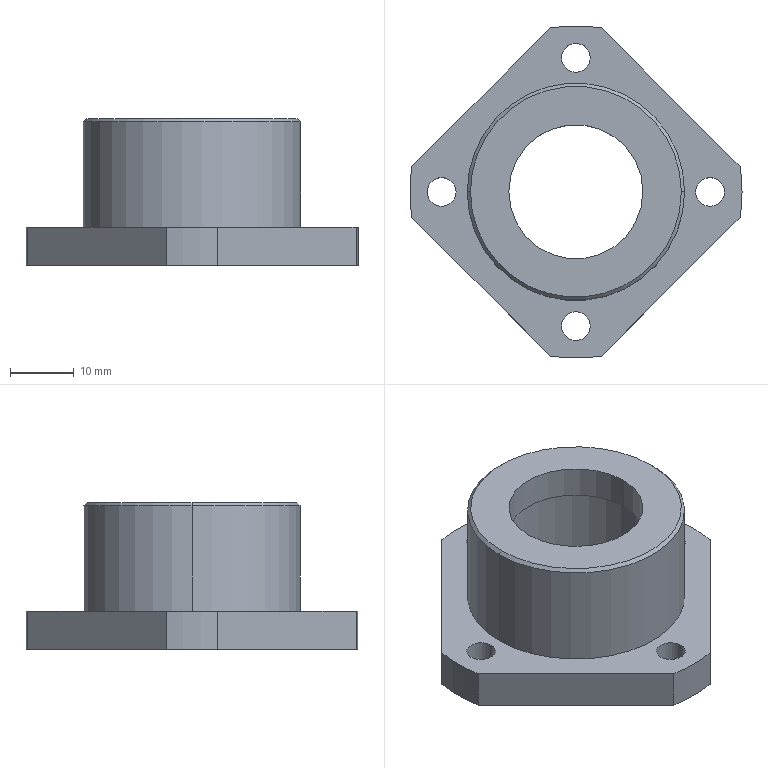Part | SolidWorks | features BaseBody 1 | 1 solid | 29 faces | box 52 x 52 x 23 mm | volume 13989 mm3 | cylinder 19 | plane 8 | cone 2 | commonest cylinder face diameters 4.5 x8 52 x5 21 x2 26 x2 34 x2
STEP:
#1=CARTESIAN_POINT('',(17.,0.,0.));
#2=VERTEX_POINT('',#1);
#3=CARTESIAN_POINT('',(-17.,0.,0.));
#4=VERTEX_POINT('',#3);
#5=CARTESIAN_POINT('',(0.,0.,0.));
#6=DIRECTION('',(0.,0.,1.));
#7=DIRECTION('',(1.,0.,0.));
#8=AXIS2_PLACEMENT_3D('',#5,#6,#7);
#9=CIRCLE('',#8,17.);
#10=EDGE_CURVE('',#2,#4,#9,.T.);
#11=ORIENTED_EDGE('',*,*,#10,.T.);
#12=CARTESIAN_POINT('',(-17.,0.,16.5));
#13=VERTEX_POINT('',#12);
#14=CARTESIAN_POINT('',(-17.,0.,-50.));
#15=DIRECTION('',(0.,0.,1.));
#16=VECTOR('',#15,1000.);
#17=LINE('',#14,#16);
#18=EDGE_CURVE('',#4,#13,#17,.T.);
#19=ORIENTED_EDGE('',*,*,#18,.T.);
#20=CARTESIAN_POINT('',(17.,0.,16.5));
#21=VERTEX_POINT('',#20);
#22=CARTESIAN_POINT('',(0.,0.,16.5));
#23=DIRECTION('',(0.,0.,-1.));
#24=DIRECTION('',(1.,0.,0.));
#25=AXIS2_PLACEMENT_3D('',#22,#23,#24);
#26=CIRCLE('',#25,17.);
#27=EDGE_CURVE('',#13,#21,#26,.T.);
#28=ORIENTED_EDGE('',*,*,#27,.T.);
#29=CARTESIAN_POINT('',(17.,0.,-50.));
#30=DIRECTION('',(0.,0.,1.));
#31=VECTOR('',#30,1000.);
#32=LINE('',#29,#31);
#33=EDGE_CURVE('',#2,#21,#32,.T.);
#34=ORIENTED_EDGE('',*,*,#33,.F.);
#35=EDGE_LOOP('',(#11,#19,#28,#34));
#36=FACE_OUTER_BOUND('',#35,.T.);
#37=CARTESIAN_POINT('',(0.,0.,-50.));
#38=DIRECTION('',(0.,0.,1.));
#39=DIRECTION('',(1.,0.,0.));
#40=AXIS2_PLACEMENT_3D('',#37,#38,#39);
#41=CYLINDRICAL_SURFACE('',#40,17.);
#42=ADVANCED_FACE('',(#36),#41,.T.);
#43=CARTESIAN_POINT('',(-16.5,0.,17.));
#44=VERTEX_POINT('',#43);
#45=CARTESIAN_POINT('',(16.5,0.,17.));
#46=VERTEX_POINT('',#45);
#47=CARTESIAN_POINT('',(0.,0.,17.));
#48=DIRECTION('',(0.,0.,-1.));
#49=DIRECTION('',(-1.,0.,0.));
#50=AXIS2_PLACEMENT_3D('',#47,#48,#49);
#51=CIRCLE('',#50,16.5);
#52=EDGE_CURVE('',#44,#46,#51,.T.);
#53=ORIENTED_EDGE('',*,*,#52,.T.);
#54=CARTESIAN_POINT('',(17.,0.,16.5));
#55=DIRECTION('',(0.7071,0.,-0.7071));
#56=VECTOR('',#55,1000.);
#57=LINE('',#54,#56);
#58=EDGE_CURVE('',#46,#21,#57,.T.);
#59=ORIENTED_EDGE('',*,*,#58,.T.);
#60=ORIENTED_EDGE('',*,*,#27,.F.);
#61=CARTESIAN_POINT('',(-17.,0.,16.5));
#62=DIRECTION('',(-0.7071,0.,-0.7071));
#63=VECTOR('',#62,1000.);
#64=LINE('',#61,#63);
#65=EDGE_CURVE('',#44,#13,#64,.T.);
#66=ORIENTED_EDGE('',*,*,#65,.F.);
#67=EDGE_LOOP('',(#53,#59,#60,#66));
#68=FACE_OUTER_BOUND('',#67,.T.);
#69=CARTESIAN_POINT('',(0.,0.,16.5));
#70=DIRECTION('',(0.,0.,-1.));
#71=DIRECTION('',(-1.,0.,0.));
#72=AXIS2_PLACEMENT_3D('',#69,#70,#71);
#73=CONICAL_SURFACE('',#72,17.,0.7854);
#74=ADVANCED_FACE('',(#68),#73,.T.);
#75=CARTESIAN_POINT('',(-2.25,-21.,0.));
#76=VERTEX_POINT('',#75);
#77=CARTESIAN_POINT('',(2.25,-21.,0.));
#78=VERTEX_POINT('',#77);
#79=CARTESIAN_POINT('',(0.,-21.,0.));
#80=DIRECTION('',(0.,0.,1.));
#81=DIRECTION('',(-1.,0.,0.));
#82=AXIS2_PLACEMENT_3D('',#79,#80,#81);
#83=CIRCLE('',#82,2.25);
#84=EDGE_CURVE('',#76,#78,#83,.T.);
#85=ORIENTED_EDGE('',*,*,#84,.T.);
#86=CARTESIAN_POINT('',(2.25,-21.,-6.));
#87=VERTEX_POINT('',#86);
#88=CARTESIAN_POINT('',(2.25,-21.,0.));
#89=DIRECTION('',(0.,0.,-1.));
#90=VECTOR('',#89,1000.);
#91=LINE('',#88,#90);
#92=EDGE_CURVE('',#78,#87,#91,.T.);
#93=ORIENTED_EDGE('',*,*,#92,.T.);
#94=CARTESIAN_POINT('',(-2.25,-21.,-6.));
#95=VERTEX_POINT('',#94);
#96=CARTESIAN_POINT('',(0.,-21.,-6.));
#97=DIRECTION('',(0.,0.,1.));
#98=DIRECTION('',(-1.,0.,0.));
#99=AXIS2_PLACEMENT_3D('',#96,#97,#98);
#100=CIRCLE('',#99,2.25);
#101=EDGE_CURVE('',#95,#87,#100,.T.);
#102=ORIENTED_EDGE('',*,*,#101,.F.);
#103=CARTESIAN_POINT('',(-2.25,-21.,0.));
#104=DIRECTION('',(0.,0.,-1.));
#105=VECTOR('',#104,1000.);
#106=LINE('',#103,#105);
#107=EDGE_CURVE('',#76,#95,#106,.T.);
#108=ORIENTED_EDGE('',*,*,#107,.F.);
#109=EDGE_LOOP('',(#85,#93,#102,#108));
#110=FACE_OUTER_BOUND('',#109,.T.);
#111=CARTESIAN_POINT('',(0.,-21.,0.));
#112=DIRECTION('',(0.,0.,-1.));
#113=DIRECTION('',(-1.,0.,0.));
#114=AXIS2_PLACEMENT_3D('',#111,#112,#113);
#115=CYLINDRICAL_SURFACE('',#114,2.25);
#116=ADVANCED_FACE('',(#110),#115,.F.);
#117=CARTESIAN_POINT('',(18.75,0.,0.));
#118=VERTEX_POINT('',#117);
#119=CARTESIAN_POINT('',(23.25,0.,0.));
#120=VERTEX_POINT('',#119);
#121=CARTESIAN_POINT('',(21.,0.,0.));
#122=DIRECTION('',(0.,0.,1.));
#123=DIRECTION('',(-1.,0.,0.));
#124=AXIS2_PLACEMENT_3D('',#121,#122,#123);
#125=CIRCLE('',#124,2.25);
#126=EDGE_CURVE('',#118,#120,#125,.T.);
#127=ORIENTED_EDGE('',*,*,#126,.T.);
#128=CARTESIAN_POINT('',(23.25,0.,-6.));
#129=VERTEX_POINT('',#128);
#130=CARTESIAN_POINT('',(23.25,0.,0.));
#131=DIRECTION('',(0.,0.,-1.));
#132=VECTOR('',#131,1000.);
#133=LINE('',#130,#132);
#134=EDGE_CURVE('',#120,#129,#133,.T.);
#135=ORIENTED_EDGE('',*,*,#134,.T.);
#136=CARTESIAN_POINT('',(18.75,0.,-6.));
#137=VERTEX_POINT('',#136);
#138=CARTESIAN_POINT('',(21.,0.,-6.));
#139=DIRECTION('',(0.,0.,1.));
#140=DIRECTION('',(-1.,0.,0.));
#141=AXIS2_PLACEMENT_3D('',#138,#139,#140);
#142=CIRCLE('',#141,2.25);
#143=EDGE_CURVE('',#137,#129,#142,.T.);
#144=ORIENTED_EDGE('',*,*,#143,.F.);
#145=CARTESIAN_POINT('',(18.75,0.,0.));
#146=DIRECTION('',(0.,0.,-1.));
#147=VECTOR('',#146,1000.);
#148=LINE('',#145,#147);
#149=EDGE_CURVE('',#118,#137,#148,.T.);
#150=ORIENTED_EDGE('',*,*,#149,.F.);
#151=EDGE_LOOP('',(#127,#135,#144,#150));
#152=FACE_OUTER_BOUND('',#151,.T.);
#153=CARTESIAN_POINT('',(21.,0.,0.));
#154=DIRECTION('',(0.,0.,-1.));
#155=DIRECTION('',(-1.,0.,0.));
#156=AXIS2_PLACEMENT_3D('',#153,#154,#155);
#157=CYLINDRICAL_SURFACE('',#156,2.25);
#158=ADVANCED_FACE('',(#152),#157,.F.);
#159=CARTESIAN_POINT('',(-23.25,0.,-6.));
#160=VERTEX_POINT('',#159);
#161=CARTESIAN_POINT('',(-18.75,0.,-6.));
#162=VERTEX_POINT('',#161);
#163=CARTESIAN_POINT('',(-21.,0.,-6.));
#164=DIRECTION('',(0.,0.,1.));
#165=DIRECTION('',(1.,0.,0.));
#166=AXIS2_PLACEMENT_3D('',#163,#164,#165);
#167=CIRCLE('',#166,2.25);
#168=EDGE_CURVE('',#160,#162,#167,.T.);
#169=ORIENTED_EDGE('',*,*,#168,.F.);
#170=CARTESIAN_POINT('',(-23.25,0.,0.));
#171=VERTEX_POINT('',#170);
#172=CARTESIAN_POINT('',(-23.25,0.,-10.));
#173=DIRECTION('',(0.,0.,1.));
#174=VECTOR('',#173,1000.);
#175=LINE('',#172,#174);
#176=EDGE_CURVE('',#160,#171,#175,.T.);
#177=ORIENTED_EDGE('',*,*,#176,.T.);
#178=CARTESIAN_POINT('',(-18.75,0.,0.));
#179=VERTEX_POINT('',#178);
#180=CARTESIAN_POINT('',(-21.,0.,0.));
#181=DIRECTION('',(0.,0.,1.));
#182=DIRECTION('',(1.,0.,0.));
#183=AXIS2_PLACEMENT_3D('',#180,#181,#182);
#184=CIRCLE('',#183,2.25);
#185=EDGE_CURVE('',#171,#179,#184,.T.);
#186=ORIENTED_EDGE('',*,*,#185,.T.);
#187=CARTESIAN_POINT('',(-18.75,0.,-10.));
#188=DIRECTION('',(0.,0.,1.));
#189=VECTOR('',#188,1000.);
#190=LINE('',#187,#189);
#191=EDGE_CURVE('',#162,#179,#190,.T.);
#192=ORIENTED_EDGE('',*,*,#191,.F.);
#193=EDGE_LOOP('',(#169,#177,#186,#192));
#194=FACE_OUTER_BOUND('',#193,.T.);
#195=CARTESIAN_POINT('',(-21.,0.,-10.));
#196=DIRECTION('',(0.,0.,1.));
#197=DIRECTION('',(1.,0.,0.));
#198=AXIS2_PLACEMENT_3D('',#195,#196,#197);
#199=CYLINDRICAL_SURFACE('',#198,2.25);
#200=ADVANCED_FACE('',(#194),#199,.F.);
#201=CARTESIAN_POINT('',(-2.25,21.,-6.));
#202=VERTEX_POINT('',#201);
#203=CARTESIAN_POINT('',(2.25,21.,-6.));
#204=VERTEX_POINT('',#203);
#205=CARTESIAN_POINT('',(0.,21.,-6.));
#206=DIRECTION('',(0.,0.,1.));
#207=DIRECTION('',(1.,0.,0.));
#208=AXIS2_PLACEMENT_3D('',#205,#206,#207);
#209=CIRCLE('',#208,2.25);
#210=EDGE_CURVE('',#202,#204,#209,.T.);
#211=ORIENTED_EDGE('',*,*,#210,.F.);
#212=CARTESIAN_POINT('',(-2.25,21.,0.));
#213=VERTEX_POINT('',#212);
#214=CARTESIAN_POINT('',(-2.25,21.,-10.));
#215=DIRECTION('',(0.,0.,1.));
#216=VECTOR('',#215,1000.);
#217=LINE('',#214,#216);
#218=EDGE_CURVE('',#202,#213,#217,.T.);
#219=ORIENTED_EDGE('',*,*,#218,.T.);
#220=CARTESIAN_POINT('',(2.25,21.,0.));
#221=VERTEX_POINT('',#220);
#222=CARTESIAN_POINT('',(0.,21.,0.));
#223=DIRECTION('',(0.,0.,1.));
#224=DIRECTION('',(1.,0.,0.));
#225=AXIS2_PLACEMENT_3D('',#222,#223,#224);
#226=CIRCLE('',#225,2.25);
#227=EDGE_CURVE('',#213,#221,#226,.T.);
#228=ORIENTED_EDGE('',*,*,#227,.T.);
#229=CARTESIAN_POINT('',(2.25,21.,-10.));
#230=DIRECTION('',(0.,0.,1.));
#231=VECTOR('',#230,1000.);
#232=LINE('',#229,#231);
#233=EDGE_CURVE('',#204,#221,#232,.T.);
#234=ORIENTED_EDGE('',*,*,#233,.F.);
#235=EDGE_LOOP('',(#211,#219,#228,#234));
#236=FACE_OUTER_BOUND('',#235,.T.);
#237=CARTESIAN_POINT('',(0.,21.,-10.));
#238=DIRECTION('',(0.,0.,1.));
#239=DIRECTION('',(1.,0.,0.));
#240=AXIS2_PLACEMENT_3D('',#237,#238,#239);
#241=CYLINDRICAL_SURFACE('',#240,2.25);
#242=ADVANCED_FACE('',(#236),#241,.F.);
#243=CARTESIAN_POINT('',(25.689,-4.01,-6.));
#244=VERTEX_POINT('',#243);
#245=CARTESIAN_POINT('',(26.,0.,-6.));
#246=VERTEX_POINT('',#245);
#247=CARTESIAN_POINT('',(0.,0.,-6.));
#248=DIRECTION('',(0.,0.,1.));
#249=DIRECTION('',(1.,0.,0.));
#250=AXIS2_PLACEMENT_3D('',#247,#248,#249);
#251=CIRCLE('',#250,26.);
#252=EDGE_CURVE('',#244,#246,#251,.T.);
#253=ORIENTED_EDGE('',*,*,#252,.T.);
#254=CARTESIAN_POINT('',(26.,0.,0.));
#255=VERTEX_POINT('',#254);
#256=CARTESIAN_POINT('',(26.,0.,-50.));
#257=DIRECTION('',(0.,0.,1.));
#258=VECTOR('',#257,1000.);
#259=LINE('',#256,#258);
#260=EDGE_CURVE('',#246,#255,#259,.T.);
#261=ORIENTED_EDGE('',*,*,#260,.T.);
#262=CARTESIAN_POINT('',(25.689,-4.01,0.));
#263=VERTEX_POINT('',#262);
#264=CARTESIAN_POINT('',(0.,0.,0.));
#265=DIRECTION('',(0.,0.,-1.));
#266=DIRECTION('',(1.,0.,0.));
#267=AXIS2_PLACEMENT_3D('',#264,#265,#266);
#268=CIRCLE('',#267,26.);
#269=EDGE_CURVE('',#255,#263,#268,.T.);
#270=ORIENTED_EDGE('',*,*,#269,.T.);
#271=CARTESIAN_POINT('',(25.689,-4.01,-10.));
#272=DIRECTION('',(0.,0.,-1.));
#273=VECTOR('',#272,1000.);
#274=LINE('',#271,#273);
#275=EDGE_CURVE('',#263,#244,#274,.T.);
#276=ORIENTED_EDGE('',*,*,#275,.T.);
#277=EDGE_LOOP('',(#253,#261,#270,#276));
#278=FACE_OUTER_BOUND('',#277,.T.);
#279=CARTESIAN_POINT('',(0.,0.,-50.));
#280=DIRECTION('',(0.,0.,1.));
#281=DIRECTION('',(1.,0.,0.));
#282=AXIS2_PLACEMENT_3D('',#279,#280,#281);
#283=CYLINDRICAL_SURFACE('',#282,26.);
#284=ADVANCED_FACE('',(#278),#283,.T.);
#285=CARTESIAN_POINT('',(-10.5,0.,12.));
#286=VERTEX_POINT('',#285);
#287=CARTESIAN_POINT('',(10.5,0.,12.));
#288=VERTEX_POINT('',#287);
#289=CARTESIAN_POINT('',(0.,0.,12.));
#290=DIRECTION('',(0.,0.,1.));
#291=DIRECTION('',(1.,0.,0.));
#292=AXIS2_PLACEMENT_3D('',#289,#290,#291);
#293=CIRCLE('',#292,10.5);
#294=EDGE_CURVE('',#286,#288,#293,.T.);
#295=ORIENTED_EDGE('',*,*,#294,.F.);
#296=CARTESIAN_POINT('',(-10.5,0.,17.));
#297=VERTEX_POINT('',#296);
#298=CARTESIAN_POINT('',(-10.5,0.,-50.));
#299=DIRECTION('',(0.,0.,1.));
#300=VECTOR('',#299,1000.);
#301=LINE('',#298,#300);
#302=EDGE_CURVE('',#286,#297,#301,.T.);
#303=ORIENTED_EDGE('',*,*,#302,.T.);
#304=CARTESIAN_POINT('',(10.5,0.,17.));
#305=VERTEX_POINT('',#304);
#306=CARTESIAN_POINT('',(0.,0.,17.));
#307=DIRECTION('',(0.,0.,1.));
#308=DIRECTION('',(1.,0.,0.));
#309=AXIS2_PLACEMENT_3D('',#306,#307,#308);
#310=CIRCLE('',#309,10.5);
#311=EDGE_CURVE('',#297,#305,#310,.T.);
#312=ORIENTED_EDGE('',*,*,#311,.T.);
#313=CARTESIAN_POINT('',(10.5,0.,-50.));
#314=DIRECTION('',(0.,0.,1.));
#315=VECTOR('',#314,1000.);
#316=LINE('',#313,#315);
#317=EDGE_CURVE('',#288,#305,#316,.T.);
#318=ORIENTED_EDGE('',*,*,#317,.F.);
#319=EDGE_LOOP('',(#295,#303,#312,#318));
#320=FACE_OUTER_BOUND('',#319,.T.);
#321=CARTESIAN_POINT('',(0.,0.,-50.));
#322=DIRECTION('',(0.,0.,1.));
#323=DIRECTION('',(1.,0.,0.));
#324=AXIS2_PLACEMENT_3D('',#321,#322,#323);
#325=CYLINDRICAL_SURFACE('',#324,10.5);
#326=ADVANCED_FACE('',(#320),#325,.F.);
#327=CARTESIAN_POINT('',(-13.,0.,-6.));
#328=VERTEX_POINT('',#327);
#329=CARTESIAN_POINT('',(13.,0.,-6.));
#330=VERTEX_POINT('',#329);
#331=CARTESIAN_POINT('',(0.,0.,-6.));
#332=DIRECTION('',(0.,0.,1.));
#333=DIRECTION('',(1.,0.,0.));
#334=AXIS2_PLACEMENT_3D('',#331,#332,#333);
#335=CIRCLE('',#334,13.);
#336=EDGE_CURVE('',#328,#330,#335,.T.);
#337=ORIENTED_EDGE('',*,*,#336,.F.);
#338=CARTESIAN_POINT('',(-13.,0.,12.));
#339=VERTEX_POINT('',#338);
#340=CARTESIAN_POINT('',(-13.,0.,-17.5));
#341=DIRECTION('',(0.,0.,1.));
#342=VECTOR('',#341,1000.);
#343=LINE('',#340,#342);
#344=EDGE_CURVE('',#328,#339,#343,.T.);
#345=ORIENTED_EDGE('',*,*,#344,.T.);
#346=CARTESIAN_POINT('',(13.,0.,12.));
#347=VERTEX_POINT('',#346);
#348=CARTESIAN_POINT('',(0.,0.,12.));
#349=DIRECTION('',(0.,0.,-1.));
#350=DIRECTION('',(1.,0.,0.));
#351=AXIS2_PLACEMENT_3D('',#348,#349,#350);
#352=CIRCLE('',#351,13.);
#353=EDGE_CURVE('',#347,#339,#352,.T.);
#354=ORIENTED_EDGE('',*,*,#353,.F.);
#355=CARTESIAN_POINT('',(13.,0.,-17.5));
#356=DIRECTION('',(0.,0.,1.));
#357=VECTOR('',#356,1000.);
#358=LINE('',#355,#357);
#359=EDGE_CURVE('',#330,#347,#358,.T.);
#360=ORIENTED_EDGE('',*,*,#359,.F.);
#361=EDGE_LOOP('',(#337,#345,#354,#360));
#362=FACE_OUTER_BOUND('',#361,.T.);
#363=CARTESIAN_POINT('',(0.,0.,-17.5));
#364=DIRECTION('',(0.,0.,1.));
#365=DIRECTION('',(1.,0.,0.));
#366=AXIS2_PLACEMENT_3D('',#363,#364,#365);
#367=CYLINDRICAL_SURFACE('',#366,13.);
#368=ADVANCED_FACE('',(#362),#367,.F.);
#369=ORIENTED_EDGE('',*,*,#18,.F.);
#370=CARTESIAN_POINT('',(0.,0.,0.));
#371=DIRECTION('',(0.,0.,1.));
#372=DIRECTION('',(1.,0.,0.));
#373=AXIS2_PLACEMENT_3D('',#370,#371,#372);
#374=CIRCLE('',#373,17.);
#375=EDGE_CURVE('',#4,#2,#374,.T.);
#376=ORIENTED_EDGE('',*,*,#375,.T.);
#377=ORIENTED_EDGE('',*,*,#33,.T.);
#378=CARTESIAN_POINT('',(0.,0.,16.5));
#379=DIRECTION('',(0.,0.,-1.));
#380=DIRECTION('',(1.,0.,0.));
#381=AXIS2_PLACEMENT_3D('',#378,#379,#380);
#382=CIRCLE('',#381,17.);
#383=EDGE_CURVE('',#21,#13,#382,.T.);
#384=ORIENTED_EDGE('',*,*,#383,.T.);
#385=EDGE_LOOP('',(#369,#376,#377,#384));
#386=FACE_OUTER_BOUND('',#385,.T.);
#387=CARTESIAN_POINT('',(0.,0.,-50.));
#388=DIRECTION('',(0.,0.,1.));
#389=DIRECTION('',(1.,0.,0.));
#390=AXIS2_PLACEMENT_3D('',#387,#388,#389);
#391=CYLINDRICAL_SURFACE('',#390,17.);
#392=ADVANCED_FACE('',(#386),#391,.T.);
#393=ORIENTED_EDGE('',*,*,#58,.F.);
#394=CARTESIAN_POINT('',(0.,0.,17.));
#395=DIRECTION('',(0.,0.,-1.));
#396=DIRECTION('',(-1.,0.,0.));
#397=AXIS2_PLACEMENT_3D('',#394,#395,#396);
#398=CIRCLE('',#397,16.5);
#399=EDGE_CURVE('',#46,#44,#398,.T.);
#400=ORIENTED_EDGE('',*,*,#399,.T.);
#401=ORIENTED_EDGE('',*,*,#65,.T.);
#402=ORIENTED_EDGE('',*,*,#383,.F.);
#403=EDGE_LOOP('',(#393,#400,#401,#402));
#404=FACE_OUTER_BOUND('',#403,.T.);
#405=CARTESIAN_POINT('',(0.,0.,16.5));
#406=DIRECTION('',(0.,0.,-1.));
#407=DIRECTION('',(-1.,0.,0.));
#408=AXIS2_PLACEMENT_3D('',#405,#406,#407);
#409=CONICAL_SURFACE('',#408,17.,0.7854);
#410=ADVANCED_FACE('',(#404),#409,.T.);
#411=ORIENTED_EDGE('',*,*,#10,.F.);
#412=ORIENTED_EDGE('',*,*,#375,.F.);
#413=EDGE_LOOP('',(#411,#412));
#414=FACE_BOUND('',#413,.T.);
#415=ORIENTED_EDGE('',*,*,#84,.F.);
#416=CARTESIAN_POINT('',(0.,-21.,0.));
#417=DIRECTION('',(0.,0.,1.));
#418=DIRECTION('',(-1.,0.,0.));
#419=AXIS2_PLACEMENT_3D('',#416,#417,#418);
#420=CIRCLE('',#419,2.25);
#421=EDGE_CURVE('',#78,#76,#420,.T.);
#422=ORIENTED_EDGE('',*,*,#421,.F.);
#423=EDGE_LOOP('',(#415,#422));
#424=FACE_BOUND('',#423,.T.);
#425=ORIENTED_EDGE('',*,*,#126,.F.);
#426=CARTESIAN_POINT('',(21.,0.,0.));
#427=DIRECTION('',(0.,0.,1.));
#428=DIRECTION('',(-1.,0.,0.));
#429=AXIS2_PLACEMENT_3D('',#426,#427,#428);
#430=CIRCLE('',#429,2.25);
#431=EDGE_CURVE('',#120,#118,#430,.T.);
#432=ORIENTED_EDGE('',*,*,#431,.F.);
#433=EDGE_LOOP('',(#425,#432));
#434=FACE_BOUND('',#433,.T.);
#435=CARTESIAN_POINT('',(-21.,0.,0.));
#436=DIRECTION('',(0.,0.,1.));
#437=DIRECTION('',(1.,0.,0.));
#438=AXIS2_PLACEMENT_3D('',#435,#436,#437);
#439=CIRCLE('',#438,2.25);
#440=EDGE_CURVE('',#179,#171,#439,.T.);
#441=ORIENTED_EDGE('',*,*,#440,.F.);
#442=ORIENTED_EDGE('',*,*,#185,.F.);
#443=EDGE_LOOP('',(#441,#442));
#444=FACE_BOUND('',#443,.T.);
#445=CARTESIAN_POINT('',(0.,21.,0.));
#446=DIRECTION('',(0.,0.,1.));
#447=DIRECTION('',(1.,0.,0.));
#448=AXIS2_PLACEMENT_3D('',#445,#446,#447);
#449=CIRCLE('',#448,2.25);
#450=EDGE_CURVE('',#221,#213,#449,.T.);
#451=ORIENTED_EDGE('',*,*,#450,.F.);
#452=ORIENTED_EDGE('',*,*,#227,.F.);
#453=EDGE_LOOP('',(#451,#452));
#454=FACE_BOUND('',#453,.T.);
#455=CARTESIAN_POINT('',(-25.689,4.01,0.));
#456=VERTEX_POINT('',#455);
#457=CARTESIAN_POINT('',(-4.01,25.689,0.));
#458=VERTEX_POINT('',#457);
#459=CARTESIAN_POINT('',(-25.689,4.01,0.));
#460=DIRECTION('',(0.7071,0.7071,0.));
#461=VECTOR('',#460,1000.);
#462=LINE('',#459,#461);
#463=EDGE_CURVE('',#456,#458,#462,.T.);
#464=ORIENTED_EDGE('',*,*,#463,.F.);
#465=CARTESIAN_POINT('',(-25.689,-4.01,0.));
#466=VERTEX_POINT('',#465);
#467=CARTESIAN_POINT('',(0.,0.,0.));
#468=DIRECTION('',(0.,0.,-1.));
#469=DIRECTION('',(1.,0.,0.));
#470=AXIS2_PLACEMENT_3D('',#467,#468,#469);
#471=CIRCLE('',#470,26.);
#472=EDGE_CURVE('',#466,#456,#471,.T.);
#473=ORIENTED_EDGE('',*,*,#472,.F.);
#474=CARTESIAN_POINT('',(-4.01,-25.689,0.));
#475=VERTEX_POINT('',#474);
#476=CARTESIAN_POINT('',(-4.01,-25.689,0.));
#477=DIRECTION('',(-0.7071,0.7071,0.));
#478=VECTOR('',#477,1000.);
#479=LINE('',#476,#478);
#480=EDGE_CURVE('',#475,#466,#479,.T.);
#481=ORIENTED_EDGE('',*,*,#480,.F.);
#482=CARTESIAN_POINT('',(4.01,-25.689,0.));
#483=VERTEX_POINT('',#482);
#484=CARTESIAN_POINT('',(0.,0.,0.));
#485=DIRECTION('',(0.,0.,-1.));
#486=DIRECTION('',(1.,0.,0.));
#487=AXIS2_PLACEMENT_3D('',#484,#485,#486);
#488=CIRCLE('',#487,26.);
#489=EDGE_CURVE('',#483,#475,#488,.T.);
#490=ORIENTED_EDGE('',*,*,#489,.F.);
#491=CARTESIAN_POINT('',(25.689,-4.01,0.));
#492=DIRECTION('',(-0.7071,-0.7071,0.));
#493=VECTOR('',#492,1000.);
#494=LINE('',#491,#493);
#495=EDGE_CURVE('',#263,#483,#494,.T.);
#496=ORIENTED_EDGE('',*,*,#495,.F.);
#497=ORIENTED_EDGE('',*,*,#269,.F.);
#498=CARTESIAN_POINT('',(25.689,4.01,0.));
#499=VERTEX_POINT('',#498);
#500=CARTESIAN_POINT('',(0.,0.,0.));
#501=DIRECTION('',(0.,0.,-1.));
#502=DIRECTION('',(1.,0.,0.));
#503=AXIS2_PLACEMENT_3D('',#500,#501,#502);
#504=CIRCLE('',#503,26.);
#505=EDGE_CURVE('',#499,#255,#504,.T.);
#506=ORIENTED_EDGE('',*,*,#505,.F.);
#507=CARTESIAN_POINT('',(4.01,25.689,0.));
#508=VERTEX_POINT('',#507);
#509=CARTESIAN_POINT('',(4.01,25.689,0.));
#510=DIRECTION('',(0.7071,-0.7071,0.));
#511=VECTOR('',#510,1000.);
#512=LINE('',#509,#511);
#513=EDGE_CURVE('',#508,#499,#512,.T.);
#514=ORIENTED_EDGE('',*,*,#513,.F.);
#515=CARTESIAN_POINT('',(0.,0.,0.));
#516=DIRECTION('',(0.,0.,-1.));
#517=DIRECTION('',(1.,0.,0.));
#518=AXIS2_PLACEMENT_3D('',#515,#516,#517);
#519=CIRCLE('',#518,26.);
#520=EDGE_CURVE('',#458,#508,#519,.T.);
#521=ORIENTED_EDGE('',*,*,#520,.F.);
#522=EDGE_LOOP('',(#464,#473,#481,#490,#496,#497,#506,#514,#521));
#523=FACE_OUTER_BOUND('',#522,.T.);
#524=CARTESIAN_POINT('',(0.,17.,0.));
#525=DIRECTION('',(0.,0.,-1.));
#526=DIRECTION('',(-1.,0.,0.));
#527=AXIS2_PLACEMENT_3D('',#524,#525,#526);
#528=PLANE('',#527);
#529=ADVANCED_FACE('',(#414,#424,#434,#444,#454,#523),#528,.F.);
#530=CARTESIAN_POINT('',(0.,0.,17.));
#531=DIRECTION('',(0.,0.,1.));
#532=DIRECTION('',(1.,0.,0.));
#533=AXIS2_PLACEMENT_3D('',#530,#531,#532);
#534=CIRCLE('',#533,10.5);
#535=EDGE_CURVE('',#305,#297,#534,.T.);
#536=ORIENTED_EDGE('',*,*,#535,.F.);
#537=ORIENTED_EDGE('',*,*,#311,.F.);
#538=EDGE_LOOP('',(#536,#537));
#539=FACE_BOUND('',#538,.T.);
#540=ORIENTED_EDGE('',*,*,#52,.F.);
#541=ORIENTED_EDGE('',*,*,#399,.F.);
#542=EDGE_LOOP('',(#540,#541));
#543=FACE_OUTER_BOUND('',#542,.T.);
#544=CARTESIAN_POINT('',(0.,10.5,17.));
#545=DIRECTION('',(0.,0.,-1.));
#546=DIRECTION('',(-1.,0.,0.));
#547=AXIS2_PLACEMENT_3D('',#544,#545,#546);
#548=PLANE('',#547);
#549=ADVANCED_FACE('',(#539,#543),#548,.F.);
#550=ORIENTED_EDGE('',*,*,#92,.F.);
#551=ORIENTED_EDGE('',*,*,#421,.T.);
#552=ORIENTED_EDGE('',*,*,#107,.T.);
#553=CARTESIAN_POINT('',(0.,-21.,-6.));
#554=DIRECTION('',(0.,0.,1.));
#555=DIRECTION('',(-1.,0.,0.));
#556=AXIS2_PLACEMENT_3D('',#553,#554,#555);
#557=CIRCLE('',#556,2.25);
#558=EDGE_CURVE('',#87,#95,#557,.T.);
#559=ORIENTED_EDGE('',*,*,#558,.F.);
#560=EDGE_LOOP('',(#550,#551,#552,#559));
#561=FACE_OUTER_BOUND('',#560,.T.);
#562=CARTESIAN_POINT('',(0.,-21.,0.));
#563=DIRECTION('',(0.,0.,-1.));
#564=DIRECTION('',(-1.,0.,0.));
#565=AXIS2_PLACEMENT_3D('',#562,#563,#564);
#566=CYLINDRICAL_SURFACE('',#565,2.25);
#567=ADVANCED_FACE('',(#561),#566,.F.);
#568=ORIENTED_EDGE('',*,*,#134,.F.);
#569=ORIENTED_EDGE('',*,*,#431,.T.);
#570=ORIENTED_EDGE('',*,*,#149,.T.);
#571=CARTESIAN_POINT('',(21.,0.,-6.));
#572=DIRECTION('',(0.,0.,1.));
#573=DIRECTION('',(-1.,0.,0.));
#574=AXIS2_PLACEMENT_3D('',#571,#572,#573);
#575=CIRCLE('',#574,2.25);
#576=EDGE_CURVE('',#129,#137,#575,.T.);
#577=ORIENTED_EDGE('',*,*,#576,.F.);
#578=EDGE_LOOP('',(#568,#569,#570,#577));
#579=FACE_OUTER_BOUND('',#578,.T.);
#580=CARTESIAN_POINT('',(21.,0.,0.));
#581=DIRECTION('',(0.,0.,-1.));
#582=DIRECTION('',(-1.,0.,0.));
#583=AXIS2_PLACEMENT_3D('',#580,#581,#582);
#584=CYLINDRICAL_SURFACE('',#583,2.25);
#585=ADVANCED_FACE('',(#579),#584,.F.);
#586=ORIENTED_EDGE('',*,*,#176,.F.);
#587=CARTESIAN_POINT('',(-21.,0.,-6.));
#588=DIRECTION('',(0.,0.,1.));
#589=DIRECTION('',(1.,0.,0.));
#590=AXIS2_PLACEMENT_3D('',#587,#588,#589);
#591=CIRCLE('',#590,2.25);
#592=EDGE_CURVE('',#162,#160,#591,.T.);
#593=ORIENTED_EDGE('',*,*,#592,.F.);
#594=ORIENTED_EDGE('',*,*,#191,.T.);
#595=ORIENTED_EDGE('',*,*,#440,.T.);
#596=EDGE_LOOP('',(#586,#593,#594,#595));
#597=FACE_OUTER_BOUND('',#596,.T.);
#598=CARTESIAN_POINT('',(-21.,0.,-10.));
#599=DIRECTION('',(0.,0.,1.));
#600=DIRECTION('',(1.,0.,0.));
#601=AXIS2_PLACEMENT_3D('',#598,#599,#600);
#602=CYLINDRICAL_SURFACE('',#601,2.25);
#603=ADVANCED_FACE('',(#597),#602,.F.);
#604=ORIENTED_EDGE('',*,*,#218,.F.);
#605=CARTESIAN_POINT('',(0.,21.,-6.));
#606=DIRECTION('',(0.,0.,1.));
#607=DIRECTION('',(1.,0.,0.));
#608=AXIS2_PLACEMENT_3D('',#605,#606,#607);
#609=CIRCLE('',#608,2.25);
#610=EDGE_CURVE('',#204,#202,#609,.T.);
#611=ORIENTED_EDGE('',*,*,#610,.F.);
#612=ORIENTED_EDGE('',*,*,#233,.T.);
#613=ORIENTED_EDGE('',*,*,#450,.T.);
#614=EDGE_LOOP('',(#604,#611,#612,#613));
#615=FACE_OUTER_BOUND('',#614,.T.);
#616=CARTESIAN_POINT('',(0.,21.,-10.));
#617=DIRECTION('',(0.,0.,1.));
#618=DIRECTION('',(1.,0.,0.));
#619=AXIS2_PLACEMENT_3D('',#616,#617,#618);
#620=CYLINDRICAL_SURFACE('',#619,2.25);
#621=ADVANCED_FACE('',(#615),#620,.F.);
#622=ORIENTED_EDGE('',*,*,#520,.T.);
#623=CARTESIAN_POINT('',(4.01,25.689,-6.));
#624=VERTEX_POINT('',#623);
#625=CARTESIAN_POINT('',(4.01,25.689,-50.));
#626=DIRECTION('',(0.,0.,-1.));
#627=VECTOR('',#626,1000.);
#628=LINE('',#625,#627);
#629=EDGE_CURVE('',#508,#624,#628,.T.);
#630=ORIENTED_EDGE('',*,*,#629,.T.);
#631=CARTESIAN_POINT('',(-4.01,25.689,-6.));
#632=VERTEX_POINT('',#631);
#633=CARTESIAN_POINT('',(0.,0.,-6.));
#634=DIRECTION('',(0.,0.,1.));
#635=DIRECTION('',(1.,0.,0.));
#636=AXIS2_PLACEMENT_3D('',#633,#634,#635);
#637=CIRCLE('',#636,26.);
#638=EDGE_CURVE('',#624,#632,#637,.T.);
#639=ORIENTED_EDGE('',*,*,#638,.T.);
#640=CARTESIAN_POINT('',(-4.01,25.689,-50.));
#641=DIRECTION('',(0.,0.,1.));
#642=VECTOR('',#641,1000.);
#643=LINE('',#640,#642);
#644=EDGE_CURVE('',#632,#458,#643,.T.);
#645=ORIENTED_EDGE('',*,*,#644,.T.);
#646=EDGE_LOOP('',(#622,#630,#639,#645));
#647=FACE_OUTER_BOUND('',#646,.T.);
#648=CARTESIAN_POINT('',(0.,0.,-50.));
#649=DIRECTION('',(0.,0.,1.));
#650=DIRECTION('',(1.,0.,0.));
#651=AXIS2_PLACEMENT_3D('',#648,#649,#650);
#652=CYLINDRICAL_SURFACE('',#651,26.);
#653=ADVANCED_FACE('',(#647),#652,.T.);
#654=CARTESIAN_POINT('',(-25.689,4.01,-6.));
#655=VERTEX_POINT('',#654);
#656=CARTESIAN_POINT('',(-25.689,4.01,-10.));
#657=DIRECTION('',(0.,0.,-1.));
#658=VECTOR('',#657,1000.);
#659=LINE('',#656,#658);
#660=EDGE_CURVE('',#456,#655,#659,.T.);
#661=ORIENTED_EDGE('',*,*,#660,.F.);
#662=ORIENTED_EDGE('',*,*,#463,.T.);
#663=ORIENTED_EDGE('',*,*,#644,.F.);
#664=CARTESIAN_POINT('',(-25.689,4.01,-6.));
#665=DIRECTION('',(0.7071,0.7071,0.));
#666=VECTOR('',#665,1000.);
#667=LINE('',#664,#666);
#668=EDGE_CURVE('',#655,#632,#667,.T.);
#669=ORIENTED_EDGE('',*,*,#668,.F.);
#670=EDGE_LOOP('',(#661,#662,#663,#669));
#671=FACE_OUTER_BOUND('',#670,.T.);
#672=CARTESIAN_POINT('',(-25.689,4.01,-10.));
#673=DIRECTION('',(0.7071,-0.7071,0.));
#674=DIRECTION('',(0.7071,0.7071,0.));
#675=AXIS2_PLACEMENT_3D('',#672,#673,#674);
#676=PLANE('',#675);
#677=ADVANCED_FACE('',(#671),#676,.F.);
#678=ORIENTED_EDGE('',*,*,#472,.T.);
#679=ORIENTED_EDGE('',*,*,#660,.T.);
#680=CARTESIAN_POINT('',(-25.689,-4.01,-6.));
#681=VERTEX_POINT('',#680);
#682=CARTESIAN_POINT('',(0.,0.,-6.));
#683=DIRECTION('',(0.,0.,1.));
#684=DIRECTION('',(1.,0.,0.));
#685=AXIS2_PLACEMENT_3D('',#682,#683,#684);
#686=CIRCLE('',#685,26.);
#687=EDGE_CURVE('',#655,#681,#686,.T.);
#688=ORIENTED_EDGE('',*,*,#687,.T.);
#689=CARTESIAN_POINT('',(-25.689,-4.01,-50.));
#690=DIRECTION('',(0.,0.,1.));
#691=VECTOR('',#690,1000.);
#692=LINE('',#689,#691);
#693=EDGE_CURVE('',#681,#466,#692,.T.);
#694=ORIENTED_EDGE('',*,*,#693,.T.);
#695=EDGE_LOOP('',(#678,#679,#688,#694));
#696=FACE_OUTER_BOUND('',#695,.T.);
#697=CARTESIAN_POINT('',(0.,0.,-50.));
#698=DIRECTION('',(0.,0.,1.));
#699=DIRECTION('',(1.,0.,0.));
#700=AXIS2_PLACEMENT_3D('',#697,#698,#699);
#701=CYLINDRICAL_SURFACE('',#700,26.);
#702=ADVANCED_FACE('',(#696),#701,.T.);
#703=CARTESIAN_POINT('',(-4.01,-25.689,-6.));
#704=VERTEX_POINT('',#703);
#705=CARTESIAN_POINT('',(-4.01,-25.689,-10.));
#706=DIRECTION('',(0.,0.,-1.));
#707=VECTOR('',#706,1000.);
#708=LINE('',#705,#707);
#709=EDGE_CURVE('',#475,#704,#708,.T.);
#710=ORIENTED_EDGE('',*,*,#709,.F.);
#711=ORIENTED_EDGE('',*,*,#480,.T.);
#712=ORIENTED_EDGE('',*,*,#693,.F.);
#713=CARTESIAN_POINT('',(-4.01,-25.689,-6.));
#714=DIRECTION('',(-0.7071,0.7071,0.));
#715=VECTOR('',#714,1000.);
#716=LINE('',#713,#715);
#717=EDGE_CURVE('',#704,#681,#716,.T.);
#718=ORIENTED_EDGE('',*,*,#717,.F.);
#719=EDGE_LOOP('',(#710,#711,#712,#718));
#720=FACE_OUTER_BOUND('',#719,.T.);
#721=CARTESIAN_POINT('',(-4.01,-25.689,-10.));
#722=DIRECTION('',(0.7071,0.7071,0.));
#723=DIRECTION('',(-0.7071,0.7071,0.));
#724=AXIS2_PLACEMENT_3D('',#721,#722,#723);
#725=PLANE('',#724);
#726=ADVANCED_FACE('',(#720),#725,.F.);
#727=ORIENTED_EDGE('',*,*,#489,.T.);
#728=ORIENTED_EDGE('',*,*,#709,.T.);
#729=CARTESIAN_POINT('',(4.01,-25.689,-6.));
#730=VERTEX_POINT('',#729);
#731=CARTESIAN_POINT('',(0.,0.,-6.));
#732=DIRECTION('',(0.,0.,1.));
#733=DIRECTION('',(1.,0.,0.));
#734=AXIS2_PLACEMENT_3D('',#731,#732,#733);
#735=CIRCLE('',#734,26.);
#736=EDGE_CURVE('',#704,#730,#735,.T.);
#737=ORIENTED_EDGE('',*,*,#736,.T.);
#738=CARTESIAN_POINT('',(4.01,-25.689,-50.));
#739=DIRECTION('',(0.,0.,1.));
#740=VECTOR('',#739,1000.);
#741=LINE('',#738,#740);
#742=EDGE_CURVE('',#730,#483,#741,.T.);
#743=ORIENTED_EDGE('',*,*,#742,.T.);
#744=EDGE_LOOP('',(#727,#728,#737,#743));
#745=FACE_OUTER_BOUND('',#744,.T.);
#746=CARTESIAN_POINT('',(0.,0.,-50.));
#747=DIRECTION('',(0.,0.,1.));
#748=DIRECTION('',(1.,0.,0.));
#749=AXIS2_PLACEMENT_3D('',#746,#747,#748);
#750=CYLINDRICAL_SURFACE('',#749,26.);
#751=ADVANCED_FACE('',(#745),#750,.T.);
#752=ORIENTED_EDGE('',*,*,#275,.F.);
#753=ORIENTED_EDGE('',*,*,#495,.T.);
#754=ORIENTED_EDGE('',*,*,#742,.F.);
#755=CARTESIAN_POINT('',(25.689,-4.01,-6.));
#756=DIRECTION('',(-0.7071,-0.7071,0.));
#757=VECTOR('',#756,1000.);
#758=LINE('',#755,#757);
#759=EDGE_CURVE('',#244,#730,#758,.T.);
#760=ORIENTED_EDGE('',*,*,#759,.F.);
#761=EDGE_LOOP('',(#752,#753,#754,#760));
#762=FACE_OUTER_BOUND('',#761,.T.);
#763=CARTESIAN_POINT('',(25.689,-4.01,-10.));
#764=DIRECTION('',(-0.7071,0.7071,0.));
#765=DIRECTION('',(-0.7071,-0.7071,0.));
#766=AXIS2_PLACEMENT_3D('',#763,#764,#765);
#767=PLANE('',#766);
#768=ADVANCED_FACE('',(#762),#767,.F.);
#769=ORIENTED_EDGE('',*,*,#260,.F.);
#770=CARTESIAN_POINT('',(25.689,4.01,-6.));
#771=VERTEX_POINT('',#770);
#772=CARTESIAN_POINT('',(0.,0.,-6.));
#773=DIRECTION('',(0.,0.,1.));
#774=DIRECTION('',(1.,0.,0.));
#775=AXIS2_PLACEMENT_3D('',#772,#773,#774);
#776=CIRCLE('',#775,26.);
#777=EDGE_CURVE('',#246,#771,#776,.T.);
#778=ORIENTED_EDGE('',*,*,#777,.T.);
#779=CARTESIAN_POINT('',(25.689,4.01,-50.));
#780=DIRECTION('',(0.,0.,1.));
#781=VECTOR('',#780,1000.);
#782=LINE('',#779,#781);
#783=EDGE_CURVE('',#771,#499,#782,.T.);
#784=ORIENTED_EDGE('',*,*,#783,.T.);
#785=ORIENTED_EDGE('',*,*,#505,.T.);
#786=EDGE_LOOP('',(#769,#778,#784,#785));
#787=FACE_OUTER_BOUND('',#786,.T.);
#788=CARTESIAN_POINT('',(0.,0.,-50.));
#789=DIRECTION('',(0.,0.,1.));
#790=DIRECTION('',(1.,0.,0.));
#791=AXIS2_PLACEMENT_3D('',#788,#789,#790);
#792=CYLINDRICAL_SURFACE('',#791,26.);
#793=ADVANCED_FACE('',(#787),#792,.T.);
#794=ORIENTED_EDGE('',*,*,#629,.F.);
#795=ORIENTED_EDGE('',*,*,#513,.T.);
#796=ORIENTED_EDGE('',*,*,#783,.F.);
#797=CARTESIAN_POINT('',(4.01,25.689,-6.));
#798=DIRECTION('',(0.7071,-0.7071,0.));
#799=VECTOR('',#798,1000.);
#800=LINE('',#797,#799);
#801=EDGE_CURVE('',#624,#771,#800,.T.);
#802=ORIENTED_EDGE('',*,*,#801,.F.);
#803=EDGE_LOOP('',(#794,#795,#796,#802));
#804=FACE_OUTER_BOUND('',#803,.T.);
#805=CARTESIAN_POINT('',(4.01,25.689,-10.));
#806=DIRECTION('',(-0.7071,-0.7071,0.));
#807=DIRECTION('',(0.7071,-0.7071,0.));
#808=AXIS2_PLACEMENT_3D('',#805,#806,#807);
#809=PLANE('',#808);
#810=ADVANCED_FACE('',(#804),#809,.F.);
#811=ORIENTED_EDGE('',*,*,#302,.F.);
#812=CARTESIAN_POINT('',(0.,0.,12.));
#813=DIRECTION('',(0.,0.,1.));
#814=DIRECTION('',(1.,0.,0.));
#815=AXIS2_PLACEMENT_3D('',#812,#813,#814);
#816=CIRCLE('',#815,10.5);
#817=EDGE_CURVE('',#288,#286,#816,.T.);
#818=ORIENTED_EDGE('',*,*,#817,.F.);
#819=ORIENTED_EDGE('',*,*,#317,.T.);
#820=ORIENTED_EDGE('',*,*,#535,.T.);
#821=EDGE_LOOP('',(#811,#818,#819,#820));
#822=FACE_OUTER_BOUND('',#821,.T.);
#823=CARTESIAN_POINT('',(0.,0.,-50.));
#824=DIRECTION('',(0.,0.,1.));
#825=DIRECTION('',(1.,0.,0.));
#826=AXIS2_PLACEMENT_3D('',#823,#824,#825);
#827=CYLINDRICAL_SURFACE('',#826,10.5);
#828=ADVANCED_FACE('',(#822),#827,.F.);
#829=ORIENTED_EDGE('',*,*,#592,.T.);
#830=ORIENTED_EDGE('',*,*,#168,.T.);
#831=EDGE_LOOP('',(#829,#830));
#832=FACE_BOUND('',#831,.T.);
#833=CARTESIAN_POINT('',(0.,0.,-6.));
#834=DIRECTION('',(0.,0.,1.));
#835=DIRECTION('',(1.,0.,0.));
#836=AXIS2_PLACEMENT_3D('',#833,#834,#835);
#837=CIRCLE('',#836,13.);
#838=EDGE_CURVE('',#330,#328,#837,.T.);
#839=ORIENTED_EDGE('',*,*,#838,.T.);
#840=ORIENTED_EDGE('',*,*,#336,.T.);
#841=EDGE_LOOP('',(#839,#840));
#842=FACE_BOUND('',#841,.T.);
#843=ORIENTED_EDGE('',*,*,#610,.T.);
#844=ORIENTED_EDGE('',*,*,#210,.T.);
#845=EDGE_LOOP('',(#843,#844));
#846=FACE_BOUND('',#845,.T.);
#847=ORIENTED_EDGE('',*,*,#717,.T.);
#848=ORIENTED_EDGE('',*,*,#687,.F.);
#849=ORIENTED_EDGE('',*,*,#668,.T.);
#850=ORIENTED_EDGE('',*,*,#638,.F.);
#851=ORIENTED_EDGE('',*,*,#801,.T.);
#852=ORIENTED_EDGE('',*,*,#777,.F.);
#853=ORIENTED_EDGE('',*,*,#252,.F.);
#854=ORIENTED_EDGE('',*,*,#759,.T.);
#855=ORIENTED_EDGE('',*,*,#736,.F.);
#856=EDGE_LOOP('',(#847,#848,#849,#850,#851,#852,#853,#854,#855));
#857=FACE_OUTER_BOUND('',#856,.T.);
#858=ORIENTED_EDGE('',*,*,#101,.T.);
#859=ORIENTED_EDGE('',*,*,#558,.T.);
#860=EDGE_LOOP('',(#858,#859));
#861=FACE_BOUND('',#860,.T.);
#862=ORIENTED_EDGE('',*,*,#143,.T.);
#863=ORIENTED_EDGE('',*,*,#576,.T.);
#864=EDGE_LOOP('',(#862,#863));
#865=FACE_BOUND('',#864,.T.);
#866=CARTESIAN_POINT('',(0.,23.25,-6.));
#867=DIRECTION('',(0.,0.,-1.));
#868=DIRECTION('',(-1.,0.,0.));
#869=AXIS2_PLACEMENT_3D('',#866,#867,#868);
#870=PLANE('',#869);
#871=ADVANCED_FACE('',(#832,#842,#846,#857,#861,#865),#870,.T.);
#872=ORIENTED_EDGE('',*,*,#817,.T.);
#873=ORIENTED_EDGE('',*,*,#294,.T.);
#874=EDGE_LOOP('',(#872,#873));
#875=FACE_BOUND('',#874,.T.);
#876=ORIENTED_EDGE('',*,*,#353,.T.);
#877=CARTESIAN_POINT('',(0.,0.,12.));
#878=DIRECTION('',(0.,0.,-1.));
#879=DIRECTION('',(1.,0.,0.));
#880=AXIS2_PLACEMENT_3D('',#877,#878,#879);
#881=CIRCLE('',#880,13.);
#882=EDGE_CURVE('',#339,#347,#881,.T.);
#883=ORIENTED_EDGE('',*,*,#882,.T.);
#884=EDGE_LOOP('',(#876,#883));
#885=FACE_OUTER_BOUND('',#884,.T.);
#886=CARTESIAN_POINT('',(0.,5.,12.));
#887=DIRECTION('',(0.,0.,-1.));
#888=DIRECTION('',(-1.,0.,0.));
#889=AXIS2_PLACEMENT_3D('',#886,#887,#888);
#890=PLANE('',#889);
#891=ADVANCED_FACE('',(#875,#885),#890,.T.);
#892=ORIENTED_EDGE('',*,*,#344,.F.);
#893=ORIENTED_EDGE('',*,*,#838,.F.);
#894=ORIENTED_EDGE('',*,*,#359,.T.);
#895=ORIENTED_EDGE('',*,*,#882,.F.);
#896=EDGE_LOOP('',(#892,#893,#894,#895));
#897=FACE_OUTER_BOUND('',#896,.T.);
#898=CARTESIAN_POINT('',(0.,0.,-17.5));
#899=DIRECTION('',(0.,0.,1.));
#900=DIRECTION('',(1.,0.,0.));
#901=AXIS2_PLACEMENT_3D('',#898,#899,#900);
#902=CYLINDRICAL_SURFACE('',#901,13.);
#903=ADVANCED_FACE('',(#897),#902,.F.);
#904=CLOSED_SHELL('',(#42,#74,#116,#158,#200,#242,#284,#326,#368,#392,#410,#529,#549,#567,#585,#603,#621,#653,#677,#702,#726,#751,#768,#793,#810,#828,#871,#891,#903));
#905=MANIFOLD_SOLID_BREP('',#904);
#906=CARTESIAN_POINT('',(0.,0.,0.));
#907=DIRECTION('',(0.,0.,1.));
#908=DIRECTION('',(1.,0.,0.));
#909=AXIS2_PLACEMENT_3D('',#906,#907,#908);
#910=(LENGTH_UNIT()NAMED_UNIT(*)SI_UNIT(.MILLI.,.METRE.));
#911=UNCERTAINTY_MEASURE_WITH_UNIT(LENGTH_MEASURE(0.00001),#910,'','');
#912=(NAMED_UNIT(*)PLANE_ANGLE_UNIT()SI_UNIT($,.RADIAN.));
#913=(NAMED_UNIT(*)SI_UNIT($,.STERADIAN.)SOLID_ANGLE_UNIT());
#914=(GEOMETRIC_REPRESENTATION_CONTEXT(3)GLOBAL_UNCERTAINTY_ASSIGNED_CONTEXT((#911))GLOBAL_UNIT_ASSIGNED_CONTEXT((#910,#912,#913))REPRESENTATION_CONTEXT('',''));
#915=ADVANCED_BREP_SHAPE_REPRESENTATION('',(#905,#909),#914);